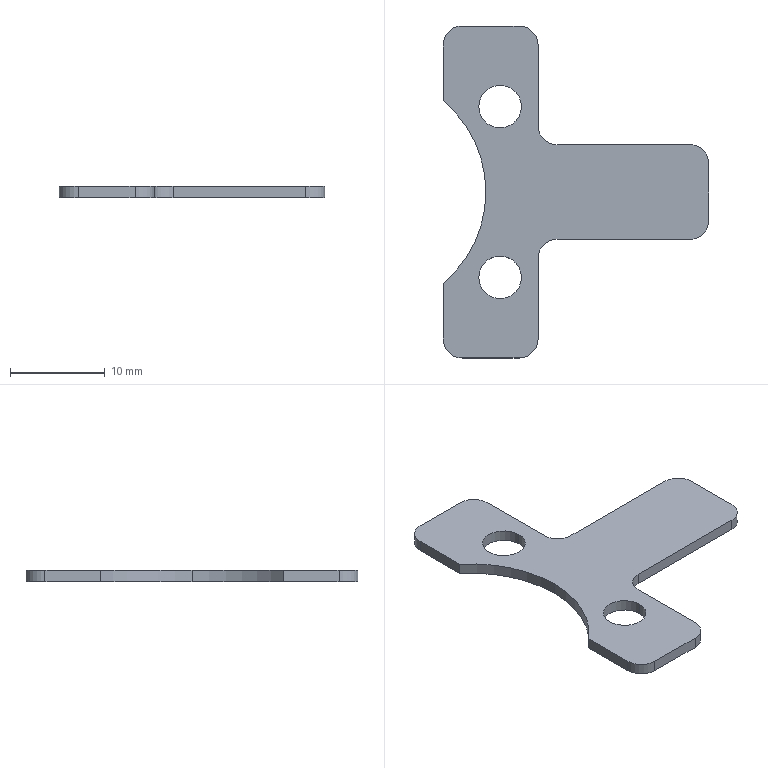Part | STEP file | 1 solid | 25 faces | box 28 x 35 x 1.2 mm | volume 521.608 mm3 | cylinder 14 | plane 11 | commonest cylinder face diameters 4 x8 4.5 x4 25 x2